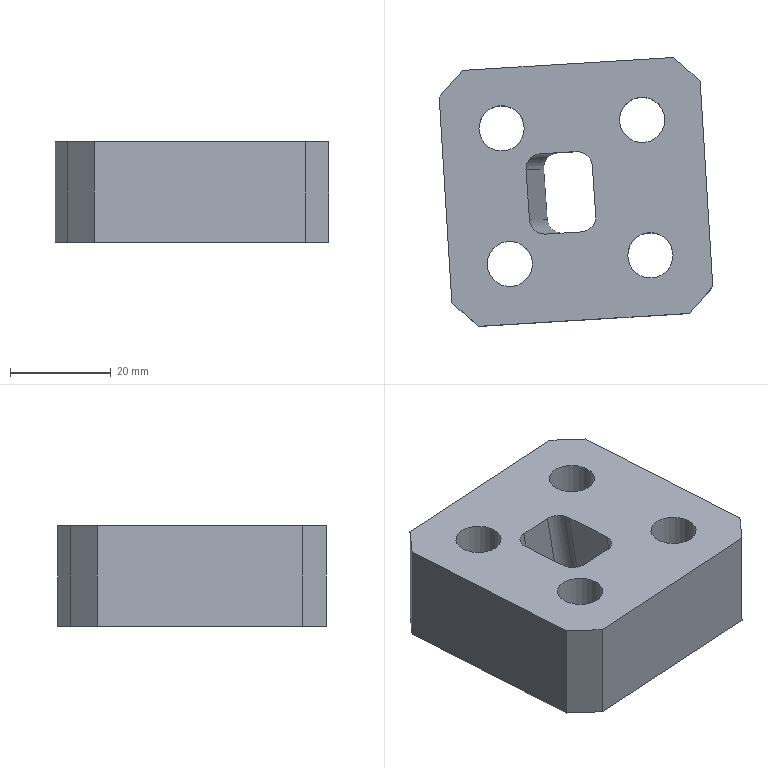Part | STEP file | 车灯-后视镜_id226_x_t | 1 solid | 30 faces | box 54.406 x 53.469 x 20 mm | volume 39812 mm3 | plane 18 | cylinder 12 | commonest cylinder face diameters 6 x4 9 x4 14 x4
STEP:
#1=CARTESIAN_POINT('',(77.366,-86.257,-160.5));
#2=VERTEX_POINT('',#1);
#3=CARTESIAN_POINT('',(70.271,-86.691,-160.5));
#4=VERTEX_POINT('',#3);
#5=CARTESIAN_POINT('',(58.281,-87.424,-160.5));
#6=DIRECTION('',(-0.9981,-0.06106,0.));
#7=VECTOR('',#6,1.);
#8=LINE('',#5,#7);
#9=EDGE_CURVE('',#2,#4,#8,.T.);
#10=ORIENTED_EDGE('',*,*,#9,.F.);
#11=CARTESIAN_POINT('',(80.222,-83.051,-160.5));
#12=VERTEX_POINT('',#11);
#13=CARTESIAN_POINT('',(77.183,-83.262,-160.5));
#14=DIRECTION('',(0.,0.,-1.));
#15=DIRECTION('',(-0.9981,-0.06106,0.));
#16=AXIS2_PLACEMENT_3D('',#13,#14,#15);
#17=ELLIPSE('',#16,3.046,3.);
#18=EDGE_CURVE('',#12,#2,#17,.T.);
#19=ORIENTED_EDGE('',*,*,#18,.F.);
#20=CARTESIAN_POINT('',(79.524,-73.074,-160.5));
#21=VERTEX_POINT('',#20);
#22=CARTESIAN_POINT('',(79.762,-76.476,-160.5));
#23=DIRECTION('',(0.06976,-0.9976,0.));
#24=VECTOR('',#23,1.);
#25=LINE('',#22,#24);
#26=EDGE_CURVE('',#21,#12,#25,.T.);
#27=ORIENTED_EDGE('',*,*,#26,.F.);
#28=CARTESIAN_POINT('',(76.302,-70.291,-160.5));
#29=VERTEX_POINT('',#28);
#30=CARTESIAN_POINT('',(76.485,-73.286,-160.5));
#31=DIRECTION('',(0.,0.,-1.));
#32=DIRECTION('',(-0.9981,-0.06106,0.));
#33=AXIS2_PLACEMENT_3D('',#30,#31,#32);
#34=ELLIPSE('',#33,3.046,3.);
#35=EDGE_CURVE('',#29,#21,#34,.T.);
#36=ORIENTED_EDGE('',*,*,#35,.F.);
#37=CARTESIAN_POINT('',(69.207,-70.725,-160.5));
#38=VERTEX_POINT('',#37);
#39=CARTESIAN_POINT('',(57.304,-71.454,-160.5));
#40=DIRECTION('',(0.9981,0.06106,0.));
#41=VECTOR('',#40,1.);
#42=LINE('',#39,#41);
#43=EDGE_CURVE('',#38,#29,#42,.T.);
#44=ORIENTED_EDGE('',*,*,#43,.F.);
#45=CARTESIAN_POINT('',(66.352,-73.931,-160.5));
#46=VERTEX_POINT('',#45);
#47=CARTESIAN_POINT('',(69.39,-73.72,-160.5));
#48=DIRECTION('',(0.,0.,-1.));
#49=DIRECTION('',(-0.9981,-0.06106,0.));
#50=AXIS2_PLACEMENT_3D('',#47,#48,#49);
#51=ELLIPSE('',#50,3.046,3.);
#52=EDGE_CURVE('',#46,#38,#51,.T.);
#53=ORIENTED_EDGE('',*,*,#52,.F.);
#54=CARTESIAN_POINT('',(67.049,-83.908,-160.5));
#55=VERTEX_POINT('',#54);
#56=CARTESIAN_POINT('',(66.594,-77.397,-160.5));
#57=DIRECTION('',(-0.06976,0.9976,0.));
#58=VECTOR('',#57,1.);
#59=LINE('',#56,#58);
#60=EDGE_CURVE('',#55,#46,#59,.T.);
#61=ORIENTED_EDGE('',*,*,#60,.F.);
#62=CARTESIAN_POINT('',(70.088,-83.696,-160.5));
#63=DIRECTION('',(0.,0.,-1.));
#64=DIRECTION('',(-0.9981,-0.06106,0.));
#65=AXIS2_PLACEMENT_3D('',#62,#63,#64);
#66=ELLIPSE('',#65,3.046,3.);
#67=EDGE_CURVE('',#4,#55,#66,.T.);
#68=ORIENTED_EDGE('',*,*,#67,.F.);
#69=EDGE_LOOP('',(#10,#19,#27,#36,#44,#53,#61,#68));
#70=FACE_BOUND('',#69,.T.);
#71=CARTESIAN_POINT('',(97.476,-56.473,-160.5));
#72=VERTEX_POINT('',#71);
#73=CARTESIAN_POINT('',(99.979,-97.396,-160.5));
#74=VERTEX_POINT('',#73);
#75=CARTESIAN_POINT('',(98.641,-75.514,-160.5));
#76=DIRECTION('',(0.06105,-0.9981,0.));
#77=VECTOR('',#76,1.);
#78=LINE('',#75,#77);
#79=EDGE_CURVE('',#72,#74,#78,.T.);
#80=ORIENTED_EDGE('',*,*,#79,.T.);
#81=CARTESIAN_POINT('',(95.294,-102.692,-160.5));
#82=VERTEX_POINT('',#81);
#83=CARTESIAN_POINT('',(91.035,-107.506,-160.5));
#84=DIRECTION('',(0.6626,0.749,0.));
#85=VECTOR('',#84,1.);
#86=LINE('',#83,#85);
#87=EDGE_CURVE('',#82,#74,#86,.T.);
#88=ORIENTED_EDGE('',*,*,#87,.F.);
#89=CARTESIAN_POINT('',(53.372,-105.256,-160.5));
#90=VERTEX_POINT('',#89);
#91=CARTESIAN_POINT('',(59.349,-104.891,-160.5));
#92=DIRECTION('',(-0.9981,-0.06105,0.));
#93=VECTOR('',#92,1.);
#94=LINE('',#91,#93);
#95=EDGE_CURVE('',#82,#90,#94,.T.);
#96=ORIENTED_EDGE('',*,*,#95,.T.);
#97=CARTESIAN_POINT('',(48.076,-100.571,-160.5));
#98=VERTEX_POINT('',#97);
#99=CARTESIAN_POINT('',(42.285,-95.447,-160.5));
#100=DIRECTION('',(0.749,-0.6626,0.));
#101=VECTOR('',#100,1.);
#102=LINE('',#99,#101);
#103=EDGE_CURVE('',#98,#90,#102,.T.);
#104=ORIENTED_EDGE('',*,*,#103,.F.);
#105=CARTESIAN_POINT('',(45.573,-59.647,-160.5));
#106=VERTEX_POINT('',#105);
#107=CARTESIAN_POINT('',(46.738,-78.689,-160.5));
#108=DIRECTION('',(-0.06105,0.9981,0.));
#109=VECTOR('',#108,1.);
#110=LINE('',#107,#109);
#111=EDGE_CURVE('',#98,#106,#110,.T.);
#112=ORIENTED_EDGE('',*,*,#111,.T.);
#113=CARTESIAN_POINT('',(50.259,-54.351,-160.5));
#114=VERTEX_POINT('',#113);
#115=CARTESIAN_POINT('',(41.783,-63.931,-160.5));
#116=DIRECTION('',(-0.6626,-0.749,0.));
#117=VECTOR('',#116,1.);
#118=LINE('',#115,#117);
#119=EDGE_CURVE('',#114,#106,#118,.T.);
#120=ORIENTED_EDGE('',*,*,#119,.F.);
#121=CARTESIAN_POINT('',(92.18,-51.787,-160.5));
#122=VERTEX_POINT('',#121);
#123=CARTESIAN_POINT('',(56.236,-53.986,-160.5));
#124=DIRECTION('',(0.9981,0.06105,0.));
#125=VECTOR('',#124,1.);
#126=LINE('',#123,#125);
#127=EDGE_CURVE('',#114,#122,#126,.T.);
#128=ORIENTED_EDGE('',*,*,#127,.T.);
#129=CARTESIAN_POINT('',(85.86,-46.195,-160.5));
#130=DIRECTION('',(-0.749,0.6626,0.));
#131=VECTOR('',#130,1.);
#132=LINE('',#129,#131);
#133=EDGE_CURVE('',#72,#122,#132,.T.);
#134=ORIENTED_EDGE('',*,*,#133,.F.);
#135=EDGE_LOOP('',(#80,#88,#96,#104,#112,#120,#128,#134));
#136=FACE_BOUND('',#135,.T.);
#137=CARTESIAN_POINT('',(52.627,-92.851,-160.5));
#138=VERTEX_POINT('',#137);
#139=CARTESIAN_POINT('',(59.627,-92.851,-160.5));
#140=DIRECTION('',(0.,0.,1.));
#141=DIRECTION('',(-1.,0.,0.));
#142=AXIS2_PLACEMENT_3D('',#139,#140,#141);
#143=CIRCLE('',#142,7.);
#144=EDGE_CURVE('',#138,#138,#143,.T.);
#145=ORIENTED_EDGE('',*,*,#144,.T.);
#146=EDGE_LOOP('',(#145));
#147=FACE_BOUND('',#146,.T.);
#148=CARTESIAN_POINT('',(80.574,-91.142,-160.5));
#149=VERTEX_POINT('',#148);
#150=CARTESIAN_POINT('',(87.574,-91.142,-160.5));
#151=DIRECTION('',(0.,0.,-1.));
#152=DIRECTION('',(-1.,0.,0.));
#153=AXIS2_PLACEMENT_3D('',#150,#151,#152);
#154=CIRCLE('',#153,7.);
#155=EDGE_CURVE('',#149,#149,#154,.T.);
#156=ORIENTED_EDGE('',*,*,#155,.F.);
#157=EDGE_LOOP('',(#156));
#158=FACE_BOUND('',#157,.T.);
#159=CARTESIAN_POINT('',(50.978,-65.902,-160.5));
#160=VERTEX_POINT('',#159);
#161=CARTESIAN_POINT('',(57.978,-65.902,-160.5));
#162=DIRECTION('',(0.,0.,-1.));
#163=DIRECTION('',(-1.,0.,0.));
#164=AXIS2_PLACEMENT_3D('',#161,#162,#163);
#165=CIRCLE('',#164,7.);
#166=EDGE_CURVE('',#160,#160,#165,.T.);
#167=ORIENTED_EDGE('',*,*,#166,.F.);
#168=EDGE_LOOP('',(#167));
#169=FACE_BOUND('',#168,.T.);
#170=CARTESIAN_POINT('',(78.926,-64.192,-160.5));
#171=VERTEX_POINT('',#170);
#172=CARTESIAN_POINT('',(85.926,-64.192,-160.5));
#173=DIRECTION('',(0.,0.,1.));
#174=DIRECTION('',(-1.,0.,0.));
#175=AXIS2_PLACEMENT_3D('',#172,#173,#174);
#176=CIRCLE('',#175,7.);
#177=EDGE_CURVE('',#171,#171,#176,.T.);
#178=ORIENTED_EDGE('',*,*,#177,.T.);
#179=EDGE_LOOP('',(#178));
#180=FACE_BOUND('',#179,.T.);
#181=CARTESIAN_POINT('',(57.706,-78.018,-160.5));
#182=DIRECTION('',(0.,0.,-1.));
#183=DIRECTION('',(0.9981,0.06105,0.));
#184=AXIS2_PLACEMENT_3D('',#181,#182,#183);
#185=PLANE('',#184);
#186=ADVANCED_FACE('',(#70,#136,#147,#158,#169,#180),#185,.T.);
#187=CARTESIAN_POINT('',(53.372,-105.256,-140.5));
#188=VERTEX_POINT('',#187);
#189=CARTESIAN_POINT('',(95.294,-102.692,-140.5));
#190=VERTEX_POINT('',#189);
#191=CARTESIAN_POINT('',(59.349,-104.891,-140.5));
#192=DIRECTION('',(0.9981,0.06105,0.));
#193=VECTOR('',#192,1.);
#194=LINE('',#191,#193);
#195=EDGE_CURVE('',#188,#190,#194,.T.);
#196=ORIENTED_EDGE('',*,*,#195,.F.);
#197=CARTESIAN_POINT('',(53.372,-105.256,-138.5));
#198=DIRECTION('',(0.,0.,1.));
#199=VECTOR('',#198,1.);
#200=LINE('',#197,#199);
#201=EDGE_CURVE('',#90,#188,#200,.T.);
#202=ORIENTED_EDGE('',*,*,#201,.F.);
#203=ORIENTED_EDGE('',*,*,#95,.F.);
#204=CARTESIAN_POINT('',(95.294,-102.692,-138.5));
#205=DIRECTION('',(0.,0.,-1.));
#206=VECTOR('',#205,1.);
#207=LINE('',#204,#206);
#208=EDGE_CURVE('',#190,#82,#207,.T.);
#209=ORIENTED_EDGE('',*,*,#208,.F.);
#210=EDGE_LOOP('',(#196,#202,#203,#209));
#211=FACE_OUTER_BOUND('',#210,.T.);
#212=CARTESIAN_POINT('',(59.349,-104.891,-138.5));
#213=DIRECTION('',(0.06105,-0.9981,0.));
#214=DIRECTION('',(0.,0.,1.));
#215=AXIS2_PLACEMENT_3D('',#212,#213,#214);
#216=PLANE('',#215);
#217=ADVANCED_FACE('',(#211),#216,.T.);
#218=ORIENTED_EDGE('',*,*,#127,.F.);
#219=CARTESIAN_POINT('',(50.259,-54.351,-140.5));
#220=VERTEX_POINT('',#219);
#221=CARTESIAN_POINT('',(50.259,-54.351,-138.5));
#222=DIRECTION('',(0.,0.,-1.));
#223=VECTOR('',#222,1.);
#224=LINE('',#221,#223);
#225=EDGE_CURVE('',#220,#114,#224,.T.);
#226=ORIENTED_EDGE('',*,*,#225,.F.);
#227=CARTESIAN_POINT('',(92.18,-51.787,-140.5));
#228=VERTEX_POINT('',#227);
#229=CARTESIAN_POINT('',(56.236,-53.986,-140.5));
#230=DIRECTION('',(-0.9981,-0.06105,0.));
#231=VECTOR('',#230,1.);
#232=LINE('',#229,#231);
#233=EDGE_CURVE('',#228,#220,#232,.T.);
#234=ORIENTED_EDGE('',*,*,#233,.F.);
#235=CARTESIAN_POINT('',(92.18,-51.787,-138.5));
#236=DIRECTION('',(0.,0.,1.));
#237=VECTOR('',#236,1.);
#238=LINE('',#235,#237);
#239=EDGE_CURVE('',#122,#228,#238,.T.);
#240=ORIENTED_EDGE('',*,*,#239,.F.);
#241=EDGE_LOOP('',(#218,#226,#234,#240));
#242=FACE_OUTER_BOUND('',#241,.T.);
#243=CARTESIAN_POINT('',(56.236,-53.986,-138.5));
#244=DIRECTION('',(-0.06105,0.9981,0.));
#245=DIRECTION('',(0.,0.,-1.));
#246=AXIS2_PLACEMENT_3D('',#243,#244,#245);
#247=PLANE('',#246);
#248=ADVANCED_FACE('',(#242),#247,.T.);
#249=CARTESIAN_POINT('',(66.751,-86.906,-140.5));
#250=VERTEX_POINT('',#249);
#251=CARTESIAN_POINT('',(73.846,-86.472,-140.5));
#252=VERTEX_POINT('',#251);
#253=CARTESIAN_POINT('',(58.281,-87.424,-140.5));
#254=DIRECTION('',(0.9981,0.06106,0.));
#255=VECTOR('',#254,1.);
#256=LINE('',#253,#255);
#257=EDGE_CURVE('',#250,#252,#256,.T.);
#258=ORIENTED_EDGE('',*,*,#257,.F.);
#259=CARTESIAN_POINT('',(63.529,-84.123,-140.5));
#260=VERTEX_POINT('',#259);
#261=CARTESIAN_POINT('',(66.568,-83.912,-140.5));
#262=DIRECTION('',(0.,0.,1.));
#263=DIRECTION('',(-0.9981,-0.06106,0.));
#264=AXIS2_PLACEMENT_3D('',#261,#262,#263);
#265=ELLIPSE('',#264,3.046,3.);
#266=EDGE_CURVE('',#260,#250,#265,.T.);
#267=ORIENTED_EDGE('',*,*,#266,.F.);
#268=CARTESIAN_POINT('',(62.831,-74.147,-140.5));
#269=VERTEX_POINT('',#268);
#270=CARTESIAN_POINT('',(63.076,-77.643,-140.5));
#271=DIRECTION('',(0.06976,-0.9976,0.));
#272=VECTOR('',#271,1.);
#273=LINE('',#270,#272);
#274=EDGE_CURVE('',#269,#260,#273,.T.);
#275=ORIENTED_EDGE('',*,*,#274,.F.);
#276=CARTESIAN_POINT('',(65.687,-70.941,-140.5));
#277=VERTEX_POINT('',#276);
#278=CARTESIAN_POINT('',(65.87,-73.935,-140.5));
#279=DIRECTION('',(0.,0.,1.));
#280=DIRECTION('',(-0.9981,-0.06106,0.));
#281=AXIS2_PLACEMENT_3D('',#278,#279,#280);
#282=ELLIPSE('',#281,3.046,3.);
#283=EDGE_CURVE('',#277,#269,#282,.T.);
#284=ORIENTED_EDGE('',*,*,#283,.F.);
#285=CARTESIAN_POINT('',(72.782,-70.507,-140.5));
#286=VERTEX_POINT('',#285);
#287=CARTESIAN_POINT('',(57.304,-71.454,-140.5));
#288=DIRECTION('',(-0.9981,-0.06106,0.));
#289=VECTOR('',#288,1.);
#290=LINE('',#287,#289);
#291=EDGE_CURVE('',#286,#277,#290,.T.);
#292=ORIENTED_EDGE('',*,*,#291,.F.);
#293=CARTESIAN_POINT('',(76.004,-73.289,-140.5));
#294=VERTEX_POINT('',#293);
#295=CARTESIAN_POINT('',(72.965,-73.501,-140.5));
#296=DIRECTION('',(0.,0.,1.));
#297=DIRECTION('',(-0.9981,-0.06106,0.));
#298=AXIS2_PLACEMENT_3D('',#295,#296,#297);
#299=ELLIPSE('',#298,3.046,3.);
#300=EDGE_CURVE('',#294,#286,#299,.T.);
#301=ORIENTED_EDGE('',*,*,#300,.F.);
#302=CARTESIAN_POINT('',(76.702,-83.266,-140.5));
#303=VERTEX_POINT('',#302);
#304=CARTESIAN_POINT('',(76.244,-76.722,-140.5));
#305=DIRECTION('',(-0.06976,0.9976,0.));
#306=VECTOR('',#305,1.);
#307=LINE('',#304,#306);
#308=EDGE_CURVE('',#303,#294,#307,.T.);
#309=ORIENTED_EDGE('',*,*,#308,.F.);
#310=CARTESIAN_POINT('',(73.663,-83.478,-140.5));
#311=DIRECTION('',(0.,0.,1.));
#312=DIRECTION('',(-0.9981,-0.06106,0.));
#313=AXIS2_PLACEMENT_3D('',#310,#311,#312);
#314=ELLIPSE('',#313,3.046,3.);
#315=EDGE_CURVE('',#252,#303,#314,.T.);
#316=ORIENTED_EDGE('',*,*,#315,.F.);
#317=EDGE_LOOP('',(#258,#267,#275,#284,#292,#301,#309,#316));
#318=FACE_BOUND('',#317,.T.);
#319=ORIENTED_EDGE('',*,*,#233,.T.);
#320=CARTESIAN_POINT('',(45.573,-59.647,-140.5));
#321=VERTEX_POINT('',#320);
#322=CARTESIAN_POINT('',(41.783,-63.931,-140.5));
#323=DIRECTION('',(0.6626,0.749,0.));
#324=VECTOR('',#323,1.);
#325=LINE('',#322,#324);
#326=EDGE_CURVE('',#321,#220,#325,.T.);
#327=ORIENTED_EDGE('',*,*,#326,.F.);
#328=CARTESIAN_POINT('',(48.076,-100.571,-140.5));
#329=VERTEX_POINT('',#328);
#330=CARTESIAN_POINT('',(46.738,-78.689,-140.5));
#331=DIRECTION('',(0.06105,-0.9981,0.));
#332=VECTOR('',#331,1.);
#333=LINE('',#330,#332);
#334=EDGE_CURVE('',#321,#329,#333,.T.);
#335=ORIENTED_EDGE('',*,*,#334,.T.);
#336=CARTESIAN_POINT('',(42.285,-95.447,-140.5));
#337=DIRECTION('',(-0.749,0.6626,0.));
#338=VECTOR('',#337,1.);
#339=LINE('',#336,#338);
#340=EDGE_CURVE('',#188,#329,#339,.T.);
#341=ORIENTED_EDGE('',*,*,#340,.F.);
#342=ORIENTED_EDGE('',*,*,#195,.T.);
#343=CARTESIAN_POINT('',(99.979,-97.396,-140.5));
#344=VERTEX_POINT('',#343);
#345=CARTESIAN_POINT('',(91.035,-107.506,-140.5));
#346=DIRECTION('',(-0.6626,-0.749,0.));
#347=VECTOR('',#346,1.);
#348=LINE('',#345,#347);
#349=EDGE_CURVE('',#344,#190,#348,.T.);
#350=ORIENTED_EDGE('',*,*,#349,.F.);
#351=CARTESIAN_POINT('',(97.476,-56.473,-140.5));
#352=VERTEX_POINT('',#351);
#353=CARTESIAN_POINT('',(98.641,-75.514,-140.5));
#354=DIRECTION('',(-0.06105,0.9981,0.));
#355=VECTOR('',#354,1.);
#356=LINE('',#353,#355);
#357=EDGE_CURVE('',#344,#352,#356,.T.);
#358=ORIENTED_EDGE('',*,*,#357,.T.);
#359=CARTESIAN_POINT('',(85.86,-46.195,-140.5));
#360=DIRECTION('',(0.749,-0.6626,0.));
#361=VECTOR('',#360,1.);
#362=LINE('',#359,#361);
#363=EDGE_CURVE('',#228,#352,#362,.T.);
#364=ORIENTED_EDGE('',*,*,#363,.F.);
#365=EDGE_LOOP('',(#319,#327,#335,#341,#342,#350,#358,#364));
#366=FACE_BOUND('',#365,.T.);
#367=CARTESIAN_POINT('',(64.127,-92.851,-140.5));
#368=VERTEX_POINT('',#367);
#369=CARTESIAN_POINT('',(59.627,-92.851,-140.5));
#370=DIRECTION('',(0.,0.,-1.));
#371=DIRECTION('',(1.,0.,0.));
#372=AXIS2_PLACEMENT_3D('',#369,#370,#371);
#373=CIRCLE('',#372,4.5);
#374=EDGE_CURVE('',#368,#368,#373,.T.);
#375=ORIENTED_EDGE('',*,*,#374,.T.);
#376=EDGE_LOOP('',(#375));
#377=FACE_BOUND('',#376,.T.);
#378=CARTESIAN_POINT('',(92.074,-91.142,-140.5));
#379=VERTEX_POINT('',#378);
#380=CARTESIAN_POINT('',(87.574,-91.142,-140.5));
#381=DIRECTION('',(0.,0.,1.));
#382=DIRECTION('',(1.,0.,0.));
#383=AXIS2_PLACEMENT_3D('',#380,#381,#382);
#384=CIRCLE('',#383,4.5);
#385=EDGE_CURVE('',#379,#379,#384,.T.);
#386=ORIENTED_EDGE('',*,*,#385,.F.);
#387=EDGE_LOOP('',(#386));
#388=FACE_BOUND('',#387,.T.);
#389=CARTESIAN_POINT('',(62.478,-65.902,-140.5));
#390=VERTEX_POINT('',#389);
#391=CARTESIAN_POINT('',(57.978,-65.902,-140.5));
#392=DIRECTION('',(0.,0.,1.));
#393=DIRECTION('',(1.,0.,0.));
#394=AXIS2_PLACEMENT_3D('',#391,#392,#393);
#395=CIRCLE('',#394,4.5);
#396=EDGE_CURVE('',#390,#390,#395,.T.);
#397=ORIENTED_EDGE('',*,*,#396,.F.);
#398=EDGE_LOOP('',(#397));
#399=FACE_BOUND('',#398,.T.);
#400=CARTESIAN_POINT('',(90.426,-64.192,-140.5));
#401=VERTEX_POINT('',#400);
#402=CARTESIAN_POINT('',(85.926,-64.192,-140.5));
#403=DIRECTION('',(0.,0.,-1.));
#404=DIRECTION('',(1.,0.,0.));
#405=AXIS2_PLACEMENT_3D('',#402,#403,#404);
#406=CIRCLE('',#405,4.5);
#407=EDGE_CURVE('',#401,#401,#406,.T.);
#408=ORIENTED_EDGE('',*,*,#407,.T.);
#409=EDGE_LOOP('',(#408));
#410=FACE_BOUND('',#409,.T.);
#411=CARTESIAN_POINT('',(57.706,-78.018,-140.5));
#412=DIRECTION('',(0.,0.,1.));
#413=DIRECTION('',(-0.9981,-0.06105,0.));
#414=AXIS2_PLACEMENT_3D('',#411,#412,#413);
#415=PLANE('',#414);
#416=ADVANCED_FACE('',(#318,#366,#377,#388,#399,#410),#415,.T.);
#417=ORIENTED_EDGE('',*,*,#357,.F.);
#418=CARTESIAN_POINT('',(99.979,-97.396,-138.5));
#419=DIRECTION('',(0.,0.,1.));
#420=VECTOR('',#419,1.);
#421=LINE('',#418,#420);
#422=EDGE_CURVE('',#74,#344,#421,.T.);
#423=ORIENTED_EDGE('',*,*,#422,.F.);
#424=ORIENTED_EDGE('',*,*,#79,.F.);
#425=CARTESIAN_POINT('',(97.476,-56.473,-138.5));
#426=DIRECTION('',(0.,0.,-1.));
#427=VECTOR('',#426,1.);
#428=LINE('',#425,#427);
#429=EDGE_CURVE('',#352,#72,#428,.T.);
#430=ORIENTED_EDGE('',*,*,#429,.F.);
#431=EDGE_LOOP('',(#417,#423,#424,#430));
#432=FACE_OUTER_BOUND('',#431,.T.);
#433=CARTESIAN_POINT('',(98.641,-75.514,-138.5));
#434=DIRECTION('',(0.9981,0.06105,0.));
#435=DIRECTION('',(0.,0.,1.));
#436=AXIS2_PLACEMENT_3D('',#433,#434,#435);
#437=PLANE('',#436);
#438=ADVANCED_FACE('',(#432),#437,.T.);
#439=CARTESIAN_POINT('',(90.426,-64.192,-152.));
#440=VERTEX_POINT('',#439);
#441=CARTESIAN_POINT('',(85.926,-64.192,-152.));
#442=DIRECTION('',(0.,0.,-1.));
#443=DIRECTION('',(1.,0.,0.));
#444=AXIS2_PLACEMENT_3D('',#441,#442,#443);
#445=CIRCLE('',#444,4.5);
#446=EDGE_CURVE('',#440,#440,#445,.T.);
#447=ORIENTED_EDGE('',*,*,#446,.T.);
#448=EDGE_LOOP('',(#447));
#449=FACE_BOUND('',#448,.T.);
#450=ORIENTED_EDGE('',*,*,#407,.F.);
#451=EDGE_LOOP('',(#450));
#452=FACE_BOUND('',#451,.T.);
#453=CARTESIAN_POINT('',(85.926,-64.192,-140.5));
#454=DIRECTION('',(0.,0.,-1.));
#455=DIRECTION('',(-0.9981,-0.06105,0.));
#456=AXIS2_PLACEMENT_3D('',#453,#454,#455);
#457=CYLINDRICAL_SURFACE('',#456,4.5);
#458=ADVANCED_FACE('',(#449,#452),#457,.F.);
#459=ORIENTED_EDGE('',*,*,#446,.F.);
#460=EDGE_LOOP('',(#459));
#461=FACE_BOUND('',#460,.T.);
#462=CARTESIAN_POINT('',(92.926,-64.192,-152.));
#463=VERTEX_POINT('',#462);
#464=CARTESIAN_POINT('',(85.926,-64.192,-152.));
#465=DIRECTION('',(0.,0.,-1.));
#466=DIRECTION('',(1.,0.,0.));
#467=AXIS2_PLACEMENT_3D('',#464,#465,#466);
#468=CIRCLE('',#467,7.);
#469=EDGE_CURVE('',#463,#463,#468,.T.);
#470=ORIENTED_EDGE('',*,*,#469,.T.);
#471=EDGE_LOOP('',(#470));
#472=FACE_BOUND('',#471,.T.);
#473=CARTESIAN_POINT('',(85.926,-64.192,-152.));
#474=DIRECTION('',(0.,0.,1.));
#475=DIRECTION('',(0.9981,0.06105,0.));
#476=AXIS2_PLACEMENT_3D('',#473,#474,#475);
#477=PLANE('',#476);
#478=ADVANCED_FACE('',(#461,#472),#477,.F.);
#479=ORIENTED_EDGE('',*,*,#469,.F.);
#480=EDGE_LOOP('',(#479));
#481=FACE_BOUND('',#480,.T.);
#482=ORIENTED_EDGE('',*,*,#177,.F.);
#483=EDGE_LOOP('',(#482));
#484=FACE_BOUND('',#483,.T.);
#485=CARTESIAN_POINT('',(85.926,-64.192,-150.5));
#486=DIRECTION('',(0.,0.,1.));
#487=DIRECTION('',(0.9981,0.06105,0.));
#488=AXIS2_PLACEMENT_3D('',#485,#486,#487);
#489=CYLINDRICAL_SURFACE('',#488,7.);
#490=ADVANCED_FACE('',(#481,#484),#489,.F.);
#491=CARTESIAN_POINT('',(62.478,-65.902,-152.));
#492=VERTEX_POINT('',#491);
#493=CARTESIAN_POINT('',(57.978,-65.902,-152.));
#494=DIRECTION('',(0.,0.,1.));
#495=DIRECTION('',(1.,0.,0.));
#496=AXIS2_PLACEMENT_3D('',#493,#494,#495);
#497=CIRCLE('',#496,4.5);
#498=EDGE_CURVE('',#492,#492,#497,.T.);
#499=ORIENTED_EDGE('',*,*,#498,.F.);
#500=EDGE_LOOP('',(#499));
#501=FACE_BOUND('',#500,.T.);
#502=ORIENTED_EDGE('',*,*,#396,.T.);
#503=EDGE_LOOP('',(#502));
#504=FACE_BOUND('',#503,.T.);
#505=CARTESIAN_POINT('',(57.978,-65.902,-140.5));
#506=DIRECTION('',(0.,0.,-1.));
#507=DIRECTION('',(0.9981,0.06105,0.));
#508=AXIS2_PLACEMENT_3D('',#505,#506,#507);
#509=CYLINDRICAL_SURFACE('',#508,4.5);
#510=ADVANCED_FACE('',(#501,#504),#509,.F.);
#511=ORIENTED_EDGE('',*,*,#498,.T.);
#512=EDGE_LOOP('',(#511));
#513=FACE_BOUND('',#512,.T.);
#514=CARTESIAN_POINT('',(64.978,-65.902,-152.));
#515=VERTEX_POINT('',#514);
#516=CARTESIAN_POINT('',(57.978,-65.902,-152.));
#517=DIRECTION('',(0.,0.,1.));
#518=DIRECTION('',(1.,0.,0.));
#519=AXIS2_PLACEMENT_3D('',#516,#517,#518);
#520=CIRCLE('',#519,7.);
#521=EDGE_CURVE('',#515,#515,#520,.T.);
#522=ORIENTED_EDGE('',*,*,#521,.F.);
#523=EDGE_LOOP('',(#522));
#524=FACE_BOUND('',#523,.T.);
#525=CARTESIAN_POINT('',(57.978,-65.902,-152.));
#526=DIRECTION('',(0.,0.,1.));
#527=DIRECTION('',(-0.9981,-0.06105,0.));
#528=AXIS2_PLACEMENT_3D('',#525,#526,#527);
#529=PLANE('',#528);
#530=ADVANCED_FACE('',(#513,#524),#529,.F.);
#531=ORIENTED_EDGE('',*,*,#521,.T.);
#532=EDGE_LOOP('',(#531));
#533=FACE_BOUND('',#532,.T.);
#534=ORIENTED_EDGE('',*,*,#166,.T.);
#535=EDGE_LOOP('',(#534));
#536=FACE_BOUND('',#535,.T.);
#537=CARTESIAN_POINT('',(57.978,-65.902,-150.5));
#538=DIRECTION('',(0.,0.,1.));
#539=DIRECTION('',(-0.9981,-0.06105,0.));
#540=AXIS2_PLACEMENT_3D('',#537,#538,#539);
#541=CYLINDRICAL_SURFACE('',#540,7.);
#542=ADVANCED_FACE('',(#533,#536),#541,.F.);
#543=CARTESIAN_POINT('',(92.074,-91.142,-152.));
#544=VERTEX_POINT('',#543);
#545=CARTESIAN_POINT('',(87.574,-91.142,-152.));
#546=DIRECTION('',(0.,0.,1.));
#547=DIRECTION('',(1.,0.,0.));
#548=AXIS2_PLACEMENT_3D('',#545,#546,#547);
#549=CIRCLE('',#548,4.5);
#550=EDGE_CURVE('',#544,#544,#549,.T.);
#551=ORIENTED_EDGE('',*,*,#550,.F.);
#552=EDGE_LOOP('',(#551));
#553=FACE_BOUND('',#552,.T.);
#554=ORIENTED_EDGE('',*,*,#385,.T.);
#555=EDGE_LOOP('',(#554));
#556=FACE_BOUND('',#555,.T.);
#557=CARTESIAN_POINT('',(87.574,-91.142,-140.5));
#558=DIRECTION('',(0.,0.,-1.));
#559=DIRECTION('',(-0.9981,-0.06105,0.));
#560=AXIS2_PLACEMENT_3D('',#557,#558,#559);
#561=CYLINDRICAL_SURFACE('',#560,4.5);
#562=ADVANCED_FACE('',(#553,#556),#561,.F.);
#563=ORIENTED_EDGE('',*,*,#550,.T.);
#564=EDGE_LOOP('',(#563));
#565=FACE_BOUND('',#564,.T.);
#566=CARTESIAN_POINT('',(94.574,-91.142,-152.));
#567=VERTEX_POINT('',#566);
#568=CARTESIAN_POINT('',(87.574,-91.142,-152.));
#569=DIRECTION('',(0.,0.,1.));
#570=DIRECTION('',(1.,0.,0.));
#571=AXIS2_PLACEMENT_3D('',#568,#569,#570);
#572=CIRCLE('',#571,7.);
#573=EDGE_CURVE('',#567,#567,#572,.T.);
#574=ORIENTED_EDGE('',*,*,#573,.F.);
#575=EDGE_LOOP('',(#574));
#576=FACE_BOUND('',#575,.T.);
#577=CARTESIAN_POINT('',(87.574,-91.142,-152.));
#578=DIRECTION('',(0.,0.,1.));
#579=DIRECTION('',(0.9981,0.06105,0.));
#580=AXIS2_PLACEMENT_3D('',#577,#578,#579);
#581=PLANE('',#580);
#582=ADVANCED_FACE('',(#565,#576),#581,.F.);
#583=ORIENTED_EDGE('',*,*,#573,.T.);
#584=EDGE_LOOP('',(#583));
#585=FACE_BOUND('',#584,.T.);
#586=ORIENTED_EDGE('',*,*,#155,.T.);
#587=EDGE_LOOP('',(#586));
#588=FACE_BOUND('',#587,.T.);
#589=CARTESIAN_POINT('',(87.574,-91.142,-150.5));
#590=DIRECTION('',(0.,0.,1.));
#591=DIRECTION('',(0.9981,0.06105,0.));
#592=AXIS2_PLACEMENT_3D('',#589,#590,#591);
#593=CYLINDRICAL_SURFACE('',#592,7.);
#594=ADVANCED_FACE('',(#585,#588),#593,.F.);
#595=CARTESIAN_POINT('',(64.127,-92.851,-152.));
#596=VERTEX_POINT('',#595);
#597=CARTESIAN_POINT('',(59.627,-92.851,-152.));
#598=DIRECTION('',(0.,0.,-1.));
#599=DIRECTION('',(1.,0.,0.));
#600=AXIS2_PLACEMENT_3D('',#597,#598,#599);
#601=CIRCLE('',#600,4.5);
#602=EDGE_CURVE('',#596,#596,#601,.T.);
#603=ORIENTED_EDGE('',*,*,#602,.T.);
#604=EDGE_LOOP('',(#603));
#605=FACE_BOUND('',#604,.T.);
#606=ORIENTED_EDGE('',*,*,#374,.F.);
#607=EDGE_LOOP('',(#606));
#608=FACE_BOUND('',#607,.T.);
#609=CARTESIAN_POINT('',(59.627,-92.851,-140.5));
#610=DIRECTION('',(0.,0.,-1.));
#611=DIRECTION('',(0.9981,0.06105,0.));
#612=AXIS2_PLACEMENT_3D('',#609,#610,#611);
#613=CYLINDRICAL_SURFACE('',#612,4.5);
#614=ADVANCED_FACE('',(#605,#608),#613,.F.);
#615=ORIENTED_EDGE('',*,*,#602,.F.);
#616=EDGE_LOOP('',(#615));
#617=FACE_BOUND('',#616,.T.);
#618=CARTESIAN_POINT('',(66.627,-92.851,-152.));
#619=VERTEX_POINT('',#618);
#620=CARTESIAN_POINT('',(59.627,-92.851,-152.));
#621=DIRECTION('',(0.,0.,-1.));
#622=DIRECTION('',(1.,0.,0.));
#623=AXIS2_PLACEMENT_3D('',#620,#621,#622);
#624=CIRCLE('',#623,7.);
#625=EDGE_CURVE('',#619,#619,#624,.T.);
#626=ORIENTED_EDGE('',*,*,#625,.T.);
#627=EDGE_LOOP('',(#626));
#628=FACE_BOUND('',#627,.T.);
#629=CARTESIAN_POINT('',(59.627,-92.851,-152.));
#630=DIRECTION('',(0.,0.,1.));
#631=DIRECTION('',(-0.9981,-0.06105,0.));
#632=AXIS2_PLACEMENT_3D('',#629,#630,#631);
#633=PLANE('',#632);
#634=ADVANCED_FACE('',(#617,#628),#633,.F.);
#635=ORIENTED_EDGE('',*,*,#625,.F.);
#636=EDGE_LOOP('',(#635));
#637=FACE_BOUND('',#636,.T.);
#638=ORIENTED_EDGE('',*,*,#144,.F.);
#639=EDGE_LOOP('',(#638));
#640=FACE_BOUND('',#639,.T.);
#641=CARTESIAN_POINT('',(59.627,-92.851,-150.5));
#642=DIRECTION('',(0.,0.,1.));
#643=DIRECTION('',(-0.9981,-0.06105,0.));
#644=AXIS2_PLACEMENT_3D('',#641,#642,#643);
#645=CYLINDRICAL_SURFACE('',#644,7.);
#646=ADVANCED_FACE('',(#637,#640),#645,.F.);
#647=ORIENTED_EDGE('',*,*,#334,.F.);
#648=CARTESIAN_POINT('',(45.573,-59.647,-144.5));
#649=DIRECTION('',(0.,0.,1.));
#650=VECTOR('',#649,1.);
#651=LINE('',#648,#650);
#652=EDGE_CURVE('',#106,#321,#651,.T.);
#653=ORIENTED_EDGE('',*,*,#652,.F.);
#654=ORIENTED_EDGE('',*,*,#111,.F.);
#655=CARTESIAN_POINT('',(48.076,-100.571,-144.5));
#656=DIRECTION('',(0.,0.,-1.));
#657=VECTOR('',#656,1.);
#658=LINE('',#655,#657);
#659=EDGE_CURVE('',#329,#98,#658,.T.);
#660=ORIENTED_EDGE('',*,*,#659,.F.);
#661=EDGE_LOOP('',(#647,#653,#654,#660));
#662=FACE_OUTER_BOUND('',#661,.T.);
#663=CARTESIAN_POINT('',(46.738,-78.689,-144.5));
#664=DIRECTION('',(0.9981,0.06105,0.));
#665=DIRECTION('',(0.,0.,-1.));
#666=AXIS2_PLACEMENT_3D('',#663,#664,#665);
#667=PLANE('',#666);
#668=ADVANCED_FACE('',(#662),#667,.F.);
#669=ORIENTED_EDGE('',*,*,#340,.T.);
#670=ORIENTED_EDGE('',*,*,#659,.T.);
#671=ORIENTED_EDGE('',*,*,#103,.T.);
#672=ORIENTED_EDGE('',*,*,#201,.T.);
#673=EDGE_LOOP('',(#669,#670,#671,#672));
#674=FACE_OUTER_BOUND('',#673,.T.);
#675=CARTESIAN_POINT('',(48.076,-100.571,-144.5));
#676=DIRECTION('',(-0.6626,-0.749,0.));
#677=DIRECTION('',(0.749,-0.6626,0.));
#678=AXIS2_PLACEMENT_3D('',#675,#676,#677);
#679=PLANE('',#678);
#680=ADVANCED_FACE('',(#674),#679,.T.);
#681=ORIENTED_EDGE('',*,*,#119,.T.);
#682=ORIENTED_EDGE('',*,*,#652,.T.);
#683=ORIENTED_EDGE('',*,*,#326,.T.);
#684=ORIENTED_EDGE('',*,*,#225,.T.);
#685=EDGE_LOOP('',(#681,#682,#683,#684));
#686=FACE_OUTER_BOUND('',#685,.T.);
#687=CARTESIAN_POINT('',(45.573,-59.647,-144.5));
#688=DIRECTION('',(-0.749,0.6626,0.));
#689=DIRECTION('',(-0.6626,-0.749,0.));
#690=AXIS2_PLACEMENT_3D('',#687,#688,#689);
#691=PLANE('',#690);
#692=ADVANCED_FACE('',(#686),#691,.T.);
#693=ORIENTED_EDGE('',*,*,#133,.T.);
#694=ORIENTED_EDGE('',*,*,#239,.T.);
#695=ORIENTED_EDGE('',*,*,#363,.T.);
#696=ORIENTED_EDGE('',*,*,#429,.T.);
#697=EDGE_LOOP('',(#693,#694,#695,#696));
#698=FACE_OUTER_BOUND('',#697,.T.);
#699=CARTESIAN_POINT('',(92.18,-51.787,-138.5));
#700=DIRECTION('',(-0.6626,-0.749,0.));
#701=DIRECTION('',(0.749,-0.6626,0.));
#702=AXIS2_PLACEMENT_3D('',#699,#700,#701);
#703=PLANE('',#702);
#704=ADVANCED_FACE('',(#698),#703,.F.);
#705=ORIENTED_EDGE('',*,*,#87,.T.);
#706=ORIENTED_EDGE('',*,*,#422,.T.);
#707=ORIENTED_EDGE('',*,*,#349,.T.);
#708=ORIENTED_EDGE('',*,*,#208,.T.);
#709=EDGE_LOOP('',(#705,#706,#707,#708));
#710=FACE_OUTER_BOUND('',#709,.T.);
#711=CARTESIAN_POINT('',(99.979,-97.396,-138.5));
#712=DIRECTION('',(-0.749,0.6626,0.));
#713=DIRECTION('',(-0.6626,-0.749,0.));
#714=AXIS2_PLACEMENT_3D('',#711,#712,#713);
#715=PLANE('',#714);
#716=ADVANCED_FACE('',(#710),#715,.F.);
#717=ORIENTED_EDGE('',*,*,#9,.T.);
#718=CARTESIAN_POINT('',(42.9,-88.365,-4.988));
#719=DIRECTION('',(0.1733,0.0106,-0.9848));
#720=VECTOR('',#719,1.);
#721=LINE('',#718,#720);
#722=EDGE_CURVE('',#250,#4,#721,.T.);
#723=ORIENTED_EDGE('',*,*,#722,.F.);
#724=ORIENTED_EDGE('',*,*,#257,.T.);
#725=CARTESIAN_POINT('',(49.781,-87.944,-3.772));
#726=DIRECTION('',(-0.1733,-0.0106,0.9848));
#727=VECTOR('',#726,1.);
#728=LINE('',#725,#727);
#729=EDGE_CURVE('',#2,#252,#728,.T.);
#730=ORIENTED_EDGE('',*,*,#729,.F.);
#731=EDGE_LOOP('',(#717,#723,#724,#730));
#732=FACE_OUTER_BOUND('',#731,.T.);
#733=CARTESIAN_POINT('',(47.609,-88.077,-4.156));
#734=DIRECTION('',(0.06106,-0.9981,0.));
#735=DIRECTION('',(0.9981,0.06106,0.));
#736=AXIS2_PLACEMENT_3D('',#733,#734,#735);
#737=PLANE('',#736);
#738=ADVANCED_FACE('',(#732),#737,.F.);
#739=ORIENTED_EDGE('',*,*,#67,.T.);
#740=CARTESIAN_POINT('',(34.073,-85.925,26.862));
#741=DIRECTION('',(-0.1733,-0.0106,0.9848));
#742=VECTOR('',#741,1.);
#743=LINE('',#740,#742);
#744=EDGE_CURVE('',#55,#260,#743,.T.);
#745=ORIENTED_EDGE('',*,*,#744,.T.);
#746=ORIENTED_EDGE('',*,*,#266,.T.);
#747=ORIENTED_EDGE('',*,*,#722,.T.);
#748=EDGE_LOOP('',(#739,#745,#746,#747));
#749=FACE_OUTER_BOUND('',#748,.T.);
#750=CARTESIAN_POINT('',(37.02,-85.719,27.383));
#751=DIRECTION('',(-0.1733,-0.0106,0.9848));
#752=DIRECTION('',(0.9849,0.,0.1733));
#753=AXIS2_PLACEMENT_3D('',#750,#751,#752);
#754=CYLINDRICAL_SURFACE('',#753,3.);
#755=ADVANCED_FACE('',(#749),#754,.F.);
#756=ORIENTED_EDGE('',*,*,#18,.T.);
#757=ORIENTED_EDGE('',*,*,#729,.T.);
#758=ORIENTED_EDGE('',*,*,#315,.T.);
#759=CARTESIAN_POINT('',(47.421,-85.057,25.863));
#760=DIRECTION('',(0.1733,0.0106,-0.9848));
#761=VECTOR('',#760,1.);
#762=LINE('',#759,#761);
#763=EDGE_CURVE('',#303,#12,#762,.T.);
#764=ORIENTED_EDGE('',*,*,#763,.T.);
#765=EDGE_LOOP('',(#756,#757,#758,#764));
#766=FACE_OUTER_BOUND('',#765,.T.);
#767=CARTESIAN_POINT('',(49.598,-84.95,-3.772));
#768=DIRECTION('',(-0.1733,-0.0106,0.9848));
#769=DIRECTION('',(0.9849,0.,0.1733));
#770=AXIS2_PLACEMENT_3D('',#767,#768,#769);
#771=CYLINDRICAL_SURFACE('',#770,3.);
#772=ADVANCED_FACE('',(#766),#771,.F.);
#773=ORIENTED_EDGE('',*,*,#26,.T.);
#774=ORIENTED_EDGE('',*,*,#763,.F.);
#775=ORIENTED_EDGE('',*,*,#308,.T.);
#776=CARTESIAN_POINT('',(46.726,-75.08,25.848));
#777=DIRECTION('',(-0.1733,-0.0106,0.9848));
#778=VECTOR('',#777,1.);
#779=LINE('',#776,#778);
#780=EDGE_CURVE('',#21,#294,#779,.T.);
#781=ORIENTED_EDGE('',*,*,#780,.F.);
#782=EDGE_LOOP('',(#773,#774,#775,#781));
#783=FACE_OUTER_BOUND('',#782,.T.);
#784=CARTESIAN_POINT('',(46.519,-72.113,25.844));
#785=DIRECTION('',(0.9824,0.0687,0.1736));
#786=DIRECTION('',(0.1741,0.,-0.9847));
#787=AXIS2_PLACEMENT_3D('',#784,#785,#786);
#788=PLANE('',#787);
#789=ADVANCED_FACE('',(#783),#788,.F.);
#790=ORIENTED_EDGE('',*,*,#35,.T.);
#791=ORIENTED_EDGE('',*,*,#780,.T.);
#792=ORIENTED_EDGE('',*,*,#300,.T.);
#793=CARTESIAN_POINT('',(48.822,-71.972,-4.367));
#794=DIRECTION('',(0.1733,0.0106,-0.9848));
#795=VECTOR('',#794,1.);
#796=LINE('',#793,#795);
#797=EDGE_CURVE('',#286,#29,#796,.T.);
#798=ORIENTED_EDGE('',*,*,#797,.T.);
#799=EDGE_LOOP('',(#790,#791,#792,#798));
#800=FACE_OUTER_BOUND('',#799,.T.);
#801=CARTESIAN_POINT('',(43.779,-75.287,25.327));
#802=DIRECTION('',(-0.1733,-0.0106,0.9848));
#803=DIRECTION('',(0.9849,0.,0.1733));
#804=AXIS2_PLACEMENT_3D('',#801,#802,#803);
#805=CYLINDRICAL_SURFACE('',#804,3.);
#806=ADVANCED_FACE('',(#800),#805,.F.);
#807=ORIENTED_EDGE('',*,*,#60,.T.);
#808=CARTESIAN_POINT('',(33.378,-75.949,26.847));
#809=DIRECTION('',(0.1733,0.0106,-0.9848));
#810=VECTOR('',#809,1.);
#811=LINE('',#808,#810);
#812=EDGE_CURVE('',#269,#46,#811,.T.);
#813=ORIENTED_EDGE('',*,*,#812,.F.);
#814=ORIENTED_EDGE('',*,*,#274,.T.);
#815=ORIENTED_EDGE('',*,*,#744,.F.);
#816=EDGE_LOOP('',(#807,#813,#814,#815));
#817=FACE_OUTER_BOUND('',#816,.T.);
#818=CARTESIAN_POINT('',(33.164,-72.881,26.843));
#819=DIRECTION('',(-0.9824,-0.0687,-0.1736));
#820=DIRECTION('',(-0.1741,0.,0.9847));
#821=AXIS2_PLACEMENT_3D('',#818,#819,#820);
#822=PLANE('',#821);
#823=ADVANCED_FACE('',(#817),#822,.F.);
#824=ORIENTED_EDGE('',*,*,#43,.T.);
#825=ORIENTED_EDGE('',*,*,#797,.F.);
#826=ORIENTED_EDGE('',*,*,#291,.T.);
#827=CARTESIAN_POINT('',(41.941,-72.393,-5.583));
#828=DIRECTION('',(-0.1733,-0.0106,0.9848));
#829=VECTOR('',#828,1.);
#830=LINE('',#827,#829);
#831=EDGE_CURVE('',#38,#277,#830,.T.);
#832=ORIENTED_EDGE('',*,*,#831,.F.);
#833=EDGE_LOOP('',(#824,#825,#826,#832));
#834=FACE_OUTER_BOUND('',#833,.T.);
#835=CARTESIAN_POINT('',(50.016,-71.899,-4.156));
#836=DIRECTION('',(-0.06106,0.9981,0.));
#837=DIRECTION('',(-0.9981,-0.06106,0.));
#838=AXIS2_PLACEMENT_3D('',#835,#836,#837);
#839=PLANE('',#838);
#840=ADVANCED_FACE('',(#834),#839,.F.);
#841=ORIENTED_EDGE('',*,*,#52,.T.);
#842=ORIENTED_EDGE('',*,*,#831,.T.);
#843=ORIENTED_EDGE('',*,*,#283,.T.);
#844=ORIENTED_EDGE('',*,*,#812,.T.);
#845=EDGE_LOOP('',(#841,#842,#843,#844));
#846=FACE_OUTER_BOUND('',#845,.T.);
#847=CARTESIAN_POINT('',(42.124,-75.388,-5.583));
#848=DIRECTION('',(-0.1733,-0.0106,0.9848));
#849=DIRECTION('',(0.9849,0.,0.1733));
#850=AXIS2_PLACEMENT_3D('',#847,#848,#849);
#851=CYLINDRICAL_SURFACE('',#850,3.);
#852=ADVANCED_FACE('',(#846),#851,.F.);
#853=CLOSED_SHELL('',(#186,#217,#248,#416,#438,#458,#478,#490,#510,#530,#542,#562,#582,#594,#614,#634,#646,#668,#680,#692,#704,#716,#738,#755,#772,#789,#806,#823,#840,#852));
#854=MANIFOLD_SOLID_BREP('',#853);
#855=(LENGTH_UNIT()NAMED_UNIT(*)SI_UNIT(.MILLI.,.METRE.));
#856=UNCERTAINTY_MEASURE_WITH_UNIT(LENGTH_MEASURE(0.00002),#855,'','');
#857=(NAMED_UNIT(*)PLANE_ANGLE_UNIT()SI_UNIT($,.RADIAN.));
#858=PLANE_ANGLE_MEASURE_WITH_UNIT(PLANE_ANGLE_MEASURE(0.01745),#857);
#859=DIMENSIONAL_EXPONENTS(0.,0.,0.,0.,0.,0.,0.);
#860=(CONVERSION_BASED_UNIT('DEGREE',#858)NAMED_UNIT(#859)PLANE_ANGLE_UNIT());
#861=(NAMED_UNIT(*)SI_UNIT($,.STERADIAN.)SOLID_ANGLE_UNIT());
#862=(GEOMETRIC_REPRESENTATION_CONTEXT(3)GLOBAL_UNCERTAINTY_ASSIGNED_CONTEXT((#856))GLOBAL_UNIT_ASSIGNED_CONTEXT((#855,#860,#861))REPRESENTATION_CONTEXT('',''));
#863=ADVANCED_BREP_SHAPE_REPRESENTATION('',(#854),#862);